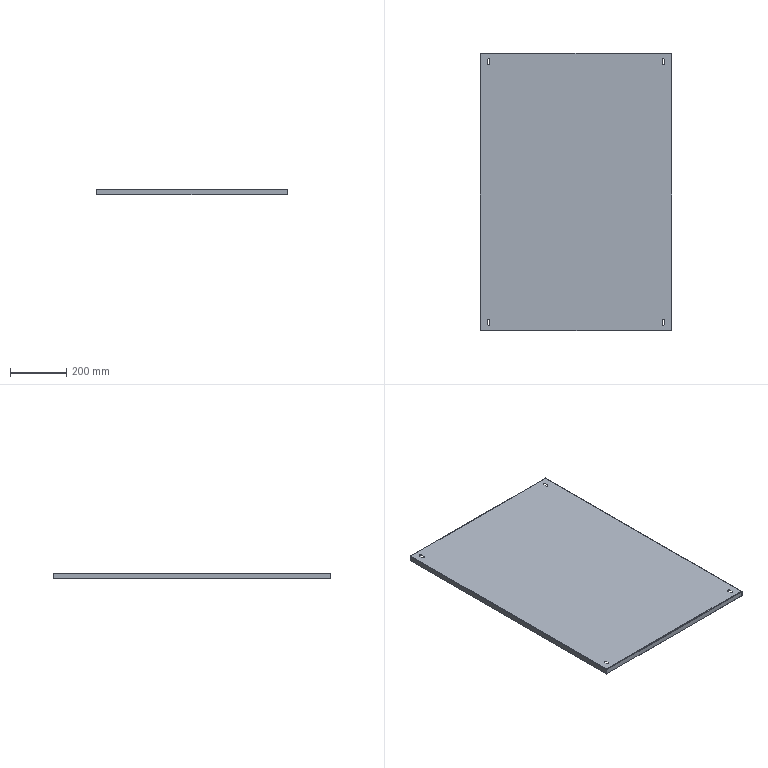Part | STEP file | Electrical Cabinet Base Plate | 1 solid | 50 faces | box 680 x 985 x 20 mm | volume 1454613 mm3 | plane 34 | cylinder 16 | commonest cylinder face diameters 10 x8 0.2 x4 4.2 x4
STEP:
#1=CARTESIAN_POINT('',(327.279,-432.271,-2.));
#2=VERTEX_POINT('',#1);
#3=CARTESIAN_POINT('',(327.279,548.529,-2.));
#4=VERTEX_POINT('',#3);
#5=CARTESIAN_POINT('',(327.279,0.,-2.));
#6=DIRECTION('',(0.,1.,0.));
#7=VECTOR('',#6,1000.);
#8=LINE('',#5,#7);
#9=EDGE_CURVE('',#2,#4,#8,.T.);
#10=ORIENTED_EDGE('',*,*,#9,.F.);
#11=CARTESIAN_POINT('',(-348.521,-432.271,-2.));
#12=VERTEX_POINT('',#11);
#13=CARTESIAN_POINT('',(0.,-432.271,-2.));
#14=DIRECTION('',(1.,0.,0.));
#15=VECTOR('',#14,1000.);
#16=LINE('',#13,#15);
#17=EDGE_CURVE('',#12,#2,#16,.T.);
#18=ORIENTED_EDGE('',*,*,#17,.F.);
#19=CARTESIAN_POINT('',(-348.521,548.529,-2.));
#20=VERTEX_POINT('',#19);
#21=CARTESIAN_POINT('',(-348.521,0.,-2.));
#22=DIRECTION('',(0.,-1.,0.));
#23=VECTOR('',#22,1000.);
#24=LINE('',#21,#23);
#25=EDGE_CURVE('',#20,#12,#24,.T.);
#26=ORIENTED_EDGE('',*,*,#25,.F.);
#27=CARTESIAN_POINT('',(0.,548.529,-2.));
#28=DIRECTION('',(-1.,0.,0.));
#29=VECTOR('',#28,1000.);
#30=LINE('',#27,#29);
#31=EDGE_CURVE('',#4,#20,#30,.T.);
#32=ORIENTED_EDGE('',*,*,#31,.F.);
#33=EDGE_LOOP('',(#10,#18,#26,#32));
#34=FACE_OUTER_BOUND('',#33,.T.);
#35=CARTESIAN_POINT('',(294.379,-399.371,-2.));
#36=VERTEX_POINT('',#35);
#37=CARTESIAN_POINT('',(304.379,-399.371,-2.));
#38=VERTEX_POINT('',#37);
#39=CARTESIAN_POINT('',(299.379,-399.371,-2.));
#40=DIRECTION('',(0.,0.,-1.));
#41=DIRECTION('',(1.,0.,0.));
#42=AXIS2_PLACEMENT_3D('',#39,#40,#41);
#43=CIRCLE('',#42,5.);
#44=EDGE_CURVE('',#36,#38,#43,.T.);
#45=ORIENTED_EDGE('',*,*,#44,.F.);
#46=CARTESIAN_POINT('',(294.379,-409.371,-2.));
#47=VERTEX_POINT('',#46);
#48=CARTESIAN_POINT('',(294.379,0.,-2.));
#49=DIRECTION('',(0.,1.,0.));
#50=VECTOR('',#49,1000.);
#51=LINE('',#48,#50);
#52=EDGE_CURVE('',#47,#36,#51,.T.);
#53=ORIENTED_EDGE('',*,*,#52,.F.);
#54=CARTESIAN_POINT('',(304.379,-409.371,-2.));
#55=VERTEX_POINT('',#54);
#56=CARTESIAN_POINT('',(299.379,-409.371,-2.));
#57=DIRECTION('',(0.,0.,-1.));
#58=DIRECTION('',(1.,0.,0.));
#59=AXIS2_PLACEMENT_3D('',#56,#57,#58);
#60=CIRCLE('',#59,5.);
#61=EDGE_CURVE('',#55,#47,#60,.T.);
#62=ORIENTED_EDGE('',*,*,#61,.F.);
#63=CARTESIAN_POINT('',(304.379,0.,-2.));
#64=DIRECTION('',(0.,-1.,0.));
#65=VECTOR('',#64,1000.);
#66=LINE('',#63,#65);
#67=EDGE_CURVE('',#38,#55,#66,.T.);
#68=ORIENTED_EDGE('',*,*,#67,.F.);
#69=EDGE_LOOP('',(#45,#53,#62,#68));
#70=FACE_BOUND('',#69,.T.);
#71=CARTESIAN_POINT('',(-325.621,-399.371,-2.));
#72=VERTEX_POINT('',#71);
#73=CARTESIAN_POINT('',(-315.621,-399.371,-2.));
#74=VERTEX_POINT('',#73);
#75=CARTESIAN_POINT('',(-320.621,-399.371,-2.));
#76=DIRECTION('',(0.,0.,-1.));
#77=DIRECTION('',(1.,0.,0.));
#78=AXIS2_PLACEMENT_3D('',#75,#76,#77);
#79=CIRCLE('',#78,5.);
#80=EDGE_CURVE('',#72,#74,#79,.T.);
#81=ORIENTED_EDGE('',*,*,#80,.F.);
#82=CARTESIAN_POINT('',(-325.621,-409.371,-2.));
#83=VERTEX_POINT('',#82);
#84=CARTESIAN_POINT('',(-325.621,0.,-2.));
#85=DIRECTION('',(0.,1.,0.));
#86=VECTOR('',#85,1000.);
#87=LINE('',#84,#86);
#88=EDGE_CURVE('',#83,#72,#87,.T.);
#89=ORIENTED_EDGE('',*,*,#88,.F.);
#90=CARTESIAN_POINT('',(-315.621,-409.371,-2.));
#91=VERTEX_POINT('',#90);
#92=CARTESIAN_POINT('',(-320.621,-409.371,-2.));
#93=DIRECTION('',(0.,0.,-1.));
#94=DIRECTION('',(1.,0.,0.));
#95=AXIS2_PLACEMENT_3D('',#92,#93,#94);
#96=CIRCLE('',#95,5.);
#97=EDGE_CURVE('',#91,#83,#96,.T.);
#98=ORIENTED_EDGE('',*,*,#97,.F.);
#99=CARTESIAN_POINT('',(-315.621,0.,-2.));
#100=DIRECTION('',(0.,-1.,0.));
#101=VECTOR('',#100,1000.);
#102=LINE('',#99,#101);
#103=EDGE_CURVE('',#74,#91,#102,.T.);
#104=ORIENTED_EDGE('',*,*,#103,.F.);
#105=EDGE_LOOP('',(#81,#89,#98,#104));
#106=FACE_BOUND('',#105,.T.);
#107=CARTESIAN_POINT('',(-325.621,525.629,-2.));
#108=VERTEX_POINT('',#107);
#109=CARTESIAN_POINT('',(-315.621,525.629,-2.));
#110=VERTEX_POINT('',#109);
#111=CARTESIAN_POINT('',(-320.621,525.629,-2.));
#112=DIRECTION('',(0.,0.,-1.));
#113=DIRECTION('',(1.,0.,0.));
#114=AXIS2_PLACEMENT_3D('',#111,#112,#113);
#115=CIRCLE('',#114,5.);
#116=EDGE_CURVE('',#108,#110,#115,.T.);
#117=ORIENTED_EDGE('',*,*,#116,.F.);
#118=CARTESIAN_POINT('',(-325.621,515.629,-2.));
#119=VERTEX_POINT('',#118);
#120=CARTESIAN_POINT('',(-325.621,0.,-2.));
#121=DIRECTION('',(0.,1.,0.));
#122=VECTOR('',#121,1000.);
#123=LINE('',#120,#122);
#124=EDGE_CURVE('',#119,#108,#123,.T.);
#125=ORIENTED_EDGE('',*,*,#124,.F.);
#126=CARTESIAN_POINT('',(-315.621,515.629,-2.));
#127=VERTEX_POINT('',#126);
#128=CARTESIAN_POINT('',(-320.621,515.629,-2.));
#129=DIRECTION('',(0.,0.,-1.));
#130=DIRECTION('',(1.,0.,0.));
#131=AXIS2_PLACEMENT_3D('',#128,#129,#130);
#132=CIRCLE('',#131,5.);
#133=EDGE_CURVE('',#127,#119,#132,.T.);
#134=ORIENTED_EDGE('',*,*,#133,.F.);
#135=CARTESIAN_POINT('',(-315.621,0.,-2.));
#136=DIRECTION('',(0.,-1.,0.));
#137=VECTOR('',#136,1000.);
#138=LINE('',#135,#137);
#139=EDGE_CURVE('',#110,#127,#138,.T.);
#140=ORIENTED_EDGE('',*,*,#139,.F.);
#141=EDGE_LOOP('',(#117,#125,#134,#140));
#142=FACE_BOUND('',#141,.T.);
#143=CARTESIAN_POINT('',(294.379,525.629,-2.));
#144=VERTEX_POINT('',#143);
#145=CARTESIAN_POINT('',(304.379,525.629,-2.));
#146=VERTEX_POINT('',#145);
#147=CARTESIAN_POINT('',(299.379,525.629,-2.));
#148=DIRECTION('',(0.,0.,-1.));
#149=DIRECTION('',(1.,0.,0.));
#150=AXIS2_PLACEMENT_3D('',#147,#148,#149);
#151=CIRCLE('',#150,5.);
#152=EDGE_CURVE('',#144,#146,#151,.T.);
#153=ORIENTED_EDGE('',*,*,#152,.F.);
#154=CARTESIAN_POINT('',(294.379,515.629,-2.));
#155=VERTEX_POINT('',#154);
#156=CARTESIAN_POINT('',(294.379,0.,-2.));
#157=DIRECTION('',(0.,1.,0.));
#158=VECTOR('',#157,1000.);
#159=LINE('',#156,#158);
#160=EDGE_CURVE('',#155,#144,#159,.T.);
#161=ORIENTED_EDGE('',*,*,#160,.F.);
#162=CARTESIAN_POINT('',(304.379,515.629,-2.));
#163=VERTEX_POINT('',#162);
#164=CARTESIAN_POINT('',(299.379,515.629,-2.));
#165=DIRECTION('',(0.,0.,-1.));
#166=DIRECTION('',(1.,0.,0.));
#167=AXIS2_PLACEMENT_3D('',#164,#165,#166);
#168=CIRCLE('',#167,5.);
#169=EDGE_CURVE('',#163,#155,#168,.T.);
#170=ORIENTED_EDGE('',*,*,#169,.F.);
#171=CARTESIAN_POINT('',(304.379,0.,-2.));
#172=DIRECTION('',(0.,-1.,0.));
#173=VECTOR('',#172,1000.);
#174=LINE('',#171,#173);
#175=EDGE_CURVE('',#146,#163,#174,.T.);
#176=ORIENTED_EDGE('',*,*,#175,.F.);
#177=EDGE_LOOP('',(#153,#161,#170,#176));
#178=FACE_BOUND('',#177,.T.);
#179=CARTESIAN_POINT('',(0.,0.,-2.));
#180=DIRECTION('',(0.,0.,1.));
#181=DIRECTION('',(1.,0.,0.));
#182=AXIS2_PLACEMENT_3D('',#179,#180,#181);
#183=PLANE('',#182);
#184=ADVANCED_FACE('',(#34,#70,#106,#142,#178),#183,.F.);
#185=CARTESIAN_POINT('',(-348.521,548.629,-2.1));
#186=VERTEX_POINT('',#185);
#187=CARTESIAN_POINT('',(-348.521,548.529,-2.1));
#188=DIRECTION('',(1.,0.,0.));
#189=DIRECTION('',(0.,0.,-1.));
#190=AXIS2_PLACEMENT_3D('',#187,#188,#189);
#191=CIRCLE('',#190,0.1);
#192=EDGE_CURVE('',#186,#20,#191,.T.);
#193=ORIENTED_EDGE('',*,*,#192,.F.);
#194=CARTESIAN_POINT('',(327.279,548.629,-2.1));
#195=VERTEX_POINT('',#194);
#196=CARTESIAN_POINT('',(327.279,548.629,-2.1));
#197=DIRECTION('',(-1.,0.,0.));
#198=VECTOR('',#197,1000.);
#199=LINE('',#196,#198);
#200=EDGE_CURVE('',#195,#186,#199,.T.);
#201=ORIENTED_EDGE('',*,*,#200,.F.);
#202=CARTESIAN_POINT('',(327.279,548.529,-2.1));
#203=DIRECTION('',(1.,0.,0.));
#204=DIRECTION('',(0.,0.,-1.));
#205=AXIS2_PLACEMENT_3D('',#202,#203,#204);
#206=CIRCLE('',#205,0.1);
#207=EDGE_CURVE('',#195,#4,#206,.T.);
#208=ORIENTED_EDGE('',*,*,#207,.T.);
#209=ORIENTED_EDGE('',*,*,#31,.T.);
#210=EDGE_LOOP('',(#193,#201,#208,#209));
#211=FACE_OUTER_BOUND('',#210,.T.);
#212=CARTESIAN_POINT('',(327.279,548.529,-2.1));
#213=DIRECTION('',(1.,0.,0.));
#214=DIRECTION('',(0.,0.,-1.));
#215=AXIS2_PLACEMENT_3D('',#212,#213,#214);
#216=CYLINDRICAL_SURFACE('',#215,0.1);
#217=ADVANCED_FACE('',(#211),#216,.F.);
#218=CARTESIAN_POINT('',(327.279,-434.369,-2.));
#219=VERTEX_POINT('',#218);
#220=CARTESIAN_POINT('',(327.279,-434.371,-2.));
#221=DIRECTION('',(0.,-1.,0.));
#222=VECTOR('',#221,1000.);
#223=LINE('',#220,#222);
#224=EDGE_CURVE('',#2,#219,#223,.T.);
#225=ORIENTED_EDGE('',*,*,#224,.F.);
#226=ORIENTED_EDGE('',*,*,#9,.T.);
#227=CARTESIAN_POINT('',(327.279,550.626,-2.));
#228=VERTEX_POINT('',#227);
#229=CARTESIAN_POINT('',(327.279,-434.371,-2.));
#230=DIRECTION('',(0.,-1.,0.));
#231=VECTOR('',#230,1000.);
#232=LINE('',#229,#231);
#233=EDGE_CURVE('',#228,#4,#232,.T.);
#234=ORIENTED_EDGE('',*,*,#233,.F.);
#235=CARTESIAN_POINT('',(327.279,550.629,-2.));
#236=VERTEX_POINT('',#235);
#237=CARTESIAN_POINT('',(327.279,550.629,-2.));
#238=DIRECTION('',(0.,-1.,0.));
#239=VECTOR('',#238,1000.);
#240=LINE('',#237,#239);
#241=EDGE_CURVE('',#236,#228,#240,.T.);
#242=ORIENTED_EDGE('',*,*,#241,.F.);
#243=CARTESIAN_POINT('',(327.379,550.629,-2.1));
#244=VERTEX_POINT('',#243);
#245=CARTESIAN_POINT('',(327.279,550.629,-2.1));
#246=DIRECTION('',(0.,-1.,0.));
#247=DIRECTION('',(0.,0.,-1.));
#248=AXIS2_PLACEMENT_3D('',#245,#246,#247);
#249=CIRCLE('',#248,0.1);
#250=EDGE_CURVE('',#244,#236,#249,.T.);
#251=ORIENTED_EDGE('',*,*,#250,.F.);
#252=CARTESIAN_POINT('',(327.379,-434.371,-2.1));
#253=VERTEX_POINT('',#252);
#254=CARTESIAN_POINT('',(327.379,-434.371,-2.1));
#255=DIRECTION('',(0.,1.,0.));
#256=VECTOR('',#255,1000.);
#257=LINE('',#254,#256);
#258=EDGE_CURVE('',#253,#244,#257,.T.);
#259=ORIENTED_EDGE('',*,*,#258,.F.);
#260=CARTESIAN_POINT('',(327.279,-434.371,-2.));
#261=VERTEX_POINT('',#260);
#262=CARTESIAN_POINT('',(327.279,-434.371,-2.1));
#263=DIRECTION('',(0.,-1.,0.));
#264=DIRECTION('',(0.,0.,-1.));
#265=AXIS2_PLACEMENT_3D('',#262,#263,#264);
#266=CIRCLE('',#265,0.1);
#267=EDGE_CURVE('',#253,#261,#266,.T.);
#268=ORIENTED_EDGE('',*,*,#267,.T.);
#269=CARTESIAN_POINT('',(327.279,-432.271,-2.));
#270=DIRECTION('',(0.,-1.,0.));
#271=VECTOR('',#270,1000.);
#272=LINE('',#269,#271);
#273=EDGE_CURVE('',#219,#261,#272,.T.);
#274=ORIENTED_EDGE('',*,*,#273,.F.);
#275=EDGE_LOOP('',(#225,#226,#234,#242,#251,#259,#268,#274));
#276=FACE_OUTER_BOUND('',#275,.T.);
#277=CARTESIAN_POINT('',(327.279,-434.371,-2.1));
#278=DIRECTION('',(0.,-1.,0.));
#279=DIRECTION('',(0.,0.,-1.));
#280=AXIS2_PLACEMENT_3D('',#277,#278,#279);
#281=CYLINDRICAL_SURFACE('',#280,0.1);
#282=ADVANCED_FACE('',(#276),#281,.F.);
#283=CARTESIAN_POINT('',(327.279,-432.371,-2.1));
#284=VERTEX_POINT('',#283);
#285=CARTESIAN_POINT('',(327.279,-432.271,-2.1));
#286=DIRECTION('',(-1.,0.,0.));
#287=DIRECTION('',(0.,0.,1.));
#288=AXIS2_PLACEMENT_3D('',#285,#286,#287);
#289=CIRCLE('',#288,0.1);
#290=EDGE_CURVE('',#284,#2,#289,.T.);
#291=ORIENTED_EDGE('',*,*,#290,.F.);
#292=CARTESIAN_POINT('',(-348.521,-432.371,-2.1));
#293=VERTEX_POINT('',#292);
#294=CARTESIAN_POINT('',(-348.521,-432.371,-2.1));
#295=DIRECTION('',(1.,0.,0.));
#296=VECTOR('',#295,1000.);
#297=LINE('',#294,#296);
#298=EDGE_CURVE('',#293,#284,#297,.T.);
#299=ORIENTED_EDGE('',*,*,#298,.F.);
#300=CARTESIAN_POINT('',(-348.521,-432.271,-2.1));
#301=DIRECTION('',(-1.,0.,0.));
#302=DIRECTION('',(0.,0.,1.));
#303=AXIS2_PLACEMENT_3D('',#300,#301,#302);
#304=CIRCLE('',#303,0.1);
#305=EDGE_CURVE('',#293,#12,#304,.T.);
#306=ORIENTED_EDGE('',*,*,#305,.T.);
#307=ORIENTED_EDGE('',*,*,#17,.T.);
#308=EDGE_LOOP('',(#291,#299,#306,#307));
#309=FACE_OUTER_BOUND('',#308,.T.);
#310=CARTESIAN_POINT('',(-348.521,-432.271,-2.1));
#311=DIRECTION('',(-1.,0.,0.));
#312=DIRECTION('',(0.,0.,1.));
#313=AXIS2_PLACEMENT_3D('',#310,#311,#312);
#314=CYLINDRICAL_SURFACE('',#313,0.1);
#315=ADVANCED_FACE('',(#309),#314,.F.);
#316=CARTESIAN_POINT('',(-348.521,550.626,-2.));
#317=VERTEX_POINT('',#316);
#318=CARTESIAN_POINT('',(-348.521,548.529,-2.));
#319=DIRECTION('',(0.,1.,0.));
#320=VECTOR('',#319,1000.);
#321=LINE('',#318,#320);
#322=EDGE_CURVE('',#20,#317,#321,.T.);
#323=ORIENTED_EDGE('',*,*,#322,.F.);
#324=ORIENTED_EDGE('',*,*,#25,.T.);
#325=CARTESIAN_POINT('',(-348.521,-434.369,-2.));
#326=VERTEX_POINT('',#325);
#327=CARTESIAN_POINT('',(-348.521,550.629,-2.));
#328=DIRECTION('',(0.,1.,0.));
#329=VECTOR('',#328,1000.);
#330=LINE('',#327,#329);
#331=EDGE_CURVE('',#326,#12,#330,.T.);
#332=ORIENTED_EDGE('',*,*,#331,.F.);
#333=CARTESIAN_POINT('',(-348.521,-434.371,-2.));
#334=VERTEX_POINT('',#333);
#335=CARTESIAN_POINT('',(-348.521,-434.371,-2.));
#336=DIRECTION('',(0.,1.,0.));
#337=VECTOR('',#336,1000.);
#338=LINE('',#335,#337);
#339=EDGE_CURVE('',#334,#326,#338,.T.);
#340=ORIENTED_EDGE('',*,*,#339,.F.);
#341=CARTESIAN_POINT('',(-348.621,-434.371,-2.1));
#342=VERTEX_POINT('',#341);
#343=CARTESIAN_POINT('',(-348.521,-434.371,-2.1));
#344=DIRECTION('',(0.,1.,0.));
#345=DIRECTION('',(0.,0.,1.));
#346=AXIS2_PLACEMENT_3D('',#343,#344,#345);
#347=CIRCLE('',#346,0.1);
#348=EDGE_CURVE('',#342,#334,#347,.T.);
#349=ORIENTED_EDGE('',*,*,#348,.F.);
#350=CARTESIAN_POINT('',(-348.621,550.629,-2.1));
#351=VERTEX_POINT('',#350);
#352=CARTESIAN_POINT('',(-348.621,550.629,-2.1));
#353=DIRECTION('',(0.,-1.,0.));
#354=VECTOR('',#353,1000.);
#355=LINE('',#352,#354);
#356=EDGE_CURVE('',#351,#342,#355,.T.);
#357=ORIENTED_EDGE('',*,*,#356,.F.);
#358=CARTESIAN_POINT('',(-348.521,550.629,-2.));
#359=VERTEX_POINT('',#358);
#360=CARTESIAN_POINT('',(-348.521,550.629,-2.1));
#361=DIRECTION('',(0.,1.,0.));
#362=DIRECTION('',(0.,0.,1.));
#363=AXIS2_PLACEMENT_3D('',#360,#361,#362);
#364=CIRCLE('',#363,0.1);
#365=EDGE_CURVE('',#351,#359,#364,.T.);
#366=ORIENTED_EDGE('',*,*,#365,.T.);
#367=CARTESIAN_POINT('',(-348.521,548.529,-2.));
#368=DIRECTION('',(0.,1.,0.));
#369=VECTOR('',#368,1000.);
#370=LINE('',#367,#369);
#371=EDGE_CURVE('',#317,#359,#370,.T.);
#372=ORIENTED_EDGE('',*,*,#371,.F.);
#373=EDGE_LOOP('',(#323,#324,#332,#340,#349,#357,#366,#372));
#374=FACE_OUTER_BOUND('',#373,.T.);
#375=CARTESIAN_POINT('',(-348.521,550.629,-2.1));
#376=DIRECTION('',(0.,1.,0.));
#377=DIRECTION('',(0.,0.,1.));
#378=AXIS2_PLACEMENT_3D('',#375,#376,#377);
#379=CYLINDRICAL_SURFACE('',#378,0.1);
#380=ADVANCED_FACE('',(#374),#379,.F.);
#381=CARTESIAN_POINT('',(304.379,-399.371,0.));
#382=VERTEX_POINT('',#381);
#383=CARTESIAN_POINT('',(304.379,-399.371,-2.));
#384=DIRECTION('',(0.,0.,1.));
#385=VECTOR('',#384,1000.);
#386=LINE('',#383,#385);
#387=EDGE_CURVE('',#38,#382,#386,.T.);
#388=ORIENTED_EDGE('',*,*,#387,.F.);
#389=ORIENTED_EDGE('',*,*,#67,.T.);
#390=CARTESIAN_POINT('',(304.379,-409.371,0.));
#391=VERTEX_POINT('',#390);
#392=CARTESIAN_POINT('',(304.379,-409.371,-2.));
#393=DIRECTION('',(0.,0.,-1.));
#394=VECTOR('',#393,1000.);
#395=LINE('',#392,#394);
#396=EDGE_CURVE('',#391,#55,#395,.T.);
#397=ORIENTED_EDGE('',*,*,#396,.F.);
#398=CARTESIAN_POINT('',(304.379,-399.371,0.));
#399=DIRECTION('',(0.,-1.,0.));
#400=VECTOR('',#399,1000.);
#401=LINE('',#398,#400);
#402=EDGE_CURVE('',#382,#391,#401,.T.);
#403=ORIENTED_EDGE('',*,*,#402,.F.);
#404=EDGE_LOOP('',(#388,#389,#397,#403));
#405=FACE_OUTER_BOUND('',#404,.T.);
#406=CARTESIAN_POINT('',(304.379,-399.371,-2.));
#407=DIRECTION('',(1.,0.,0.));
#408=DIRECTION('',(0.,0.,-1.));
#409=AXIS2_PLACEMENT_3D('',#406,#407,#408);
#410=PLANE('',#409);
#411=ADVANCED_FACE('',(#405),#410,.F.);
#412=CARTESIAN_POINT('',(294.379,-399.371,0.));
#413=VERTEX_POINT('',#412);
#414=CARTESIAN_POINT('',(294.379,-399.371,-2.));
#415=DIRECTION('',(0.,0.,1.));
#416=VECTOR('',#415,1000.);
#417=LINE('',#414,#416);
#418=EDGE_CURVE('',#36,#413,#417,.T.);
#419=ORIENTED_EDGE('',*,*,#418,.F.);
#420=ORIENTED_EDGE('',*,*,#44,.T.);
#421=ORIENTED_EDGE('',*,*,#387,.T.);
#422=CARTESIAN_POINT('',(299.379,-399.371,0.));
#423=DIRECTION('',(0.,0.,-1.));
#424=DIRECTION('',(1.,0.,0.));
#425=AXIS2_PLACEMENT_3D('',#422,#423,#424);
#426=CIRCLE('',#425,5.);
#427=EDGE_CURVE('',#413,#382,#426,.T.);
#428=ORIENTED_EDGE('',*,*,#427,.F.);
#429=EDGE_LOOP('',(#419,#420,#421,#428));
#430=FACE_OUTER_BOUND('',#429,.T.);
#431=CARTESIAN_POINT('',(299.379,-399.371,-2.));
#432=DIRECTION('',(0.,0.,1.));
#433=DIRECTION('',(1.,0.,0.));
#434=AXIS2_PLACEMENT_3D('',#431,#432,#433);
#435=CYLINDRICAL_SURFACE('',#434,5.);
#436=ADVANCED_FACE('',(#430),#435,.F.);
#437=CARTESIAN_POINT('',(294.379,-409.371,0.));
#438=VERTEX_POINT('',#437);
#439=CARTESIAN_POINT('',(294.379,-409.371,-2.));
#440=DIRECTION('',(0.,0.,1.));
#441=VECTOR('',#440,1000.);
#442=LINE('',#439,#441);
#443=EDGE_CURVE('',#47,#438,#442,.T.);
#444=ORIENTED_EDGE('',*,*,#443,.F.);
#445=ORIENTED_EDGE('',*,*,#52,.T.);
#446=ORIENTED_EDGE('',*,*,#418,.T.);
#447=CARTESIAN_POINT('',(294.379,-399.371,0.));
#448=DIRECTION('',(0.,1.,0.));
#449=VECTOR('',#448,1000.);
#450=LINE('',#447,#449);
#451=EDGE_CURVE('',#438,#413,#450,.T.);
#452=ORIENTED_EDGE('',*,*,#451,.F.);
#453=EDGE_LOOP('',(#444,#445,#446,#452));
#454=FACE_OUTER_BOUND('',#453,.T.);
#455=CARTESIAN_POINT('',(294.379,-399.371,-2.));
#456=DIRECTION('',(-1.,0.,0.));
#457=DIRECTION('',(0.,0.,1.));
#458=AXIS2_PLACEMENT_3D('',#455,#456,#457);
#459=PLANE('',#458);
#460=ADVANCED_FACE('',(#454),#459,.F.);
#461=ORIENTED_EDGE('',*,*,#396,.T.);
#462=ORIENTED_EDGE('',*,*,#61,.T.);
#463=ORIENTED_EDGE('',*,*,#443,.T.);
#464=CARTESIAN_POINT('',(299.379,-409.371,0.));
#465=DIRECTION('',(0.,0.,-1.));
#466=DIRECTION('',(1.,0.,0.));
#467=AXIS2_PLACEMENT_3D('',#464,#465,#466);
#468=CIRCLE('',#467,5.);
#469=EDGE_CURVE('',#391,#438,#468,.T.);
#470=ORIENTED_EDGE('',*,*,#469,.F.);
#471=EDGE_LOOP('',(#461,#462,#463,#470));
#472=FACE_OUTER_BOUND('',#471,.T.);
#473=CARTESIAN_POINT('',(299.379,-409.371,-2.));
#474=DIRECTION('',(0.,0.,1.));
#475=DIRECTION('',(1.,0.,0.));
#476=AXIS2_PLACEMENT_3D('',#473,#474,#475);
#477=CYLINDRICAL_SURFACE('',#476,5.);
#478=ADVANCED_FACE('',(#472),#477,.F.);
#479=CARTESIAN_POINT('',(-315.621,-399.371,0.));
#480=VERTEX_POINT('',#479);
#481=CARTESIAN_POINT('',(-315.621,-399.371,-2.));
#482=DIRECTION('',(0.,0.,1.));
#483=VECTOR('',#482,1000.);
#484=LINE('',#481,#483);
#485=EDGE_CURVE('',#74,#480,#484,.T.);
#486=ORIENTED_EDGE('',*,*,#485,.F.);
#487=ORIENTED_EDGE('',*,*,#103,.T.);
#488=CARTESIAN_POINT('',(-315.621,-409.371,0.));
#489=VERTEX_POINT('',#488);
#490=CARTESIAN_POINT('',(-315.621,-409.371,-2.));
#491=DIRECTION('',(0.,0.,-1.));
#492=VECTOR('',#491,1000.);
#493=LINE('',#490,#492);
#494=EDGE_CURVE('',#489,#91,#493,.T.);
#495=ORIENTED_EDGE('',*,*,#494,.F.);
#496=CARTESIAN_POINT('',(-315.621,-399.371,0.));
#497=DIRECTION('',(0.,-1.,0.));
#498=VECTOR('',#497,1000.);
#499=LINE('',#496,#498);
#500=EDGE_CURVE('',#480,#489,#499,.T.);
#501=ORIENTED_EDGE('',*,*,#500,.F.);
#502=EDGE_LOOP('',(#486,#487,#495,#501));
#503=FACE_OUTER_BOUND('',#502,.T.);
#504=CARTESIAN_POINT('',(-315.621,-399.371,-2.));
#505=DIRECTION('',(1.,0.,0.));
#506=DIRECTION('',(0.,0.,-1.));
#507=AXIS2_PLACEMENT_3D('',#504,#505,#506);
#508=PLANE('',#507);
#509=ADVANCED_FACE('',(#503),#508,.F.);
#510=CARTESIAN_POINT('',(-325.621,-399.371,0.));
#511=VERTEX_POINT('',#510);
#512=CARTESIAN_POINT('',(-325.621,-399.371,-2.));
#513=DIRECTION('',(0.,0.,1.));
#514=VECTOR('',#513,1000.);
#515=LINE('',#512,#514);
#516=EDGE_CURVE('',#72,#511,#515,.T.);
#517=ORIENTED_EDGE('',*,*,#516,.F.);
#518=ORIENTED_EDGE('',*,*,#80,.T.);
#519=ORIENTED_EDGE('',*,*,#485,.T.);
#520=CARTESIAN_POINT('',(-320.621,-399.371,0.));
#521=DIRECTION('',(0.,0.,-1.));
#522=DIRECTION('',(1.,0.,0.));
#523=AXIS2_PLACEMENT_3D('',#520,#521,#522);
#524=CIRCLE('',#523,5.);
#525=EDGE_CURVE('',#511,#480,#524,.T.);
#526=ORIENTED_EDGE('',*,*,#525,.F.);
#527=EDGE_LOOP('',(#517,#518,#519,#526));
#528=FACE_OUTER_BOUND('',#527,.T.);
#529=CARTESIAN_POINT('',(-320.621,-399.371,-2.));
#530=DIRECTION('',(0.,0.,1.));
#531=DIRECTION('',(1.,0.,0.));
#532=AXIS2_PLACEMENT_3D('',#529,#530,#531);
#533=CYLINDRICAL_SURFACE('',#532,5.);
#534=ADVANCED_FACE('',(#528),#533,.F.);
#535=CARTESIAN_POINT('',(-325.621,-409.371,0.));
#536=VERTEX_POINT('',#535);
#537=CARTESIAN_POINT('',(-325.621,-409.371,-2.));
#538=DIRECTION('',(0.,0.,1.));
#539=VECTOR('',#538,1000.);
#540=LINE('',#537,#539);
#541=EDGE_CURVE('',#83,#536,#540,.T.);
#542=ORIENTED_EDGE('',*,*,#541,.F.);
#543=ORIENTED_EDGE('',*,*,#88,.T.);
#544=ORIENTED_EDGE('',*,*,#516,.T.);
#545=CARTESIAN_POINT('',(-325.621,-399.371,0.));
#546=DIRECTION('',(0.,1.,0.));
#547=VECTOR('',#546,1000.);
#548=LINE('',#545,#547);
#549=EDGE_CURVE('',#536,#511,#548,.T.);
#550=ORIENTED_EDGE('',*,*,#549,.F.);
#551=EDGE_LOOP('',(#542,#543,#544,#550));
#552=FACE_OUTER_BOUND('',#551,.T.);
#553=CARTESIAN_POINT('',(-325.621,-399.371,-2.));
#554=DIRECTION('',(-1.,0.,0.));
#555=DIRECTION('',(0.,0.,1.));
#556=AXIS2_PLACEMENT_3D('',#553,#554,#555);
#557=PLANE('',#556);
#558=ADVANCED_FACE('',(#552),#557,.F.);
#559=ORIENTED_EDGE('',*,*,#494,.T.);
#560=ORIENTED_EDGE('',*,*,#97,.T.);
#561=ORIENTED_EDGE('',*,*,#541,.T.);
#562=CARTESIAN_POINT('',(-320.621,-409.371,0.));
#563=DIRECTION('',(0.,0.,-1.));
#564=DIRECTION('',(1.,0.,0.));
#565=AXIS2_PLACEMENT_3D('',#562,#563,#564);
#566=CIRCLE('',#565,5.);
#567=EDGE_CURVE('',#489,#536,#566,.T.);
#568=ORIENTED_EDGE('',*,*,#567,.F.);
#569=EDGE_LOOP('',(#559,#560,#561,#568));
#570=FACE_OUTER_BOUND('',#569,.T.);
#571=CARTESIAN_POINT('',(-320.621,-409.371,-2.));
#572=DIRECTION('',(0.,0.,1.));
#573=DIRECTION('',(1.,0.,0.));
#574=AXIS2_PLACEMENT_3D('',#571,#572,#573);
#575=CYLINDRICAL_SURFACE('',#574,5.);
#576=ADVANCED_FACE('',(#570),#575,.F.);
#577=CARTESIAN_POINT('',(-315.621,525.629,0.));
#578=VERTEX_POINT('',#577);
#579=CARTESIAN_POINT('',(-315.621,525.629,-2.));
#580=DIRECTION('',(0.,0.,1.));
#581=VECTOR('',#580,1000.);
#582=LINE('',#579,#581);
#583=EDGE_CURVE('',#110,#578,#582,.T.);
#584=ORIENTED_EDGE('',*,*,#583,.F.);
#585=ORIENTED_EDGE('',*,*,#139,.T.);
#586=CARTESIAN_POINT('',(-315.621,515.629,0.));
#587=VERTEX_POINT('',#586);
#588=CARTESIAN_POINT('',(-315.621,515.629,-2.));
#589=DIRECTION('',(0.,0.,-1.));
#590=VECTOR('',#589,1000.);
#591=LINE('',#588,#590);
#592=EDGE_CURVE('',#587,#127,#591,.T.);
#593=ORIENTED_EDGE('',*,*,#592,.F.);
#594=CARTESIAN_POINT('',(-315.621,525.629,0.));
#595=DIRECTION('',(0.,-1.,0.));
#596=VECTOR('',#595,1000.);
#597=LINE('',#594,#596);
#598=EDGE_CURVE('',#578,#587,#597,.T.);
#599=ORIENTED_EDGE('',*,*,#598,.F.);
#600=EDGE_LOOP('',(#584,#585,#593,#599));
#601=FACE_OUTER_BOUND('',#600,.T.);
#602=CARTESIAN_POINT('',(-315.621,525.629,-2.));
#603=DIRECTION('',(1.,0.,0.));
#604=DIRECTION('',(0.,0.,-1.));
#605=AXIS2_PLACEMENT_3D('',#602,#603,#604);
#606=PLANE('',#605);
#607=ADVANCED_FACE('',(#601),#606,.F.);
#608=CARTESIAN_POINT('',(-325.621,525.629,0.));
#609=VERTEX_POINT('',#608);
#610=CARTESIAN_POINT('',(-325.621,525.629,-2.));
#611=DIRECTION('',(0.,0.,1.));
#612=VECTOR('',#611,1000.);
#613=LINE('',#610,#612);
#614=EDGE_CURVE('',#108,#609,#613,.T.);
#615=ORIENTED_EDGE('',*,*,#614,.F.);
#616=ORIENTED_EDGE('',*,*,#116,.T.);
#617=ORIENTED_EDGE('',*,*,#583,.T.);
#618=CARTESIAN_POINT('',(-320.621,525.629,0.));
#619=DIRECTION('',(0.,0.,-1.));
#620=DIRECTION('',(1.,0.,0.));
#621=AXIS2_PLACEMENT_3D('',#618,#619,#620);
#622=CIRCLE('',#621,5.);
#623=EDGE_CURVE('',#609,#578,#622,.T.);
#624=ORIENTED_EDGE('',*,*,#623,.F.);
#625=EDGE_LOOP('',(#615,#616,#617,#624));
#626=FACE_OUTER_BOUND('',#625,.T.);
#627=CARTESIAN_POINT('',(-320.621,525.629,-2.));
#628=DIRECTION('',(0.,0.,1.));
#629=DIRECTION('',(1.,0.,0.));
#630=AXIS2_PLACEMENT_3D('',#627,#628,#629);
#631=CYLINDRICAL_SURFACE('',#630,5.);
#632=ADVANCED_FACE('',(#626),#631,.F.);
#633=CARTESIAN_POINT('',(-325.621,515.629,0.));
#634=VERTEX_POINT('',#633);
#635=CARTESIAN_POINT('',(-325.621,515.629,-2.));
#636=DIRECTION('',(0.,0.,1.));
#637=VECTOR('',#636,1000.);
#638=LINE('',#635,#637);
#639=EDGE_CURVE('',#119,#634,#638,.T.);
#640=ORIENTED_EDGE('',*,*,#639,.F.);
#641=ORIENTED_EDGE('',*,*,#124,.T.);
#642=ORIENTED_EDGE('',*,*,#614,.T.);
#643=CARTESIAN_POINT('',(-325.621,525.629,0.));
#644=DIRECTION('',(0.,1.,0.));
#645=VECTOR('',#644,1000.);
#646=LINE('',#643,#645);
#647=EDGE_CURVE('',#634,#609,#646,.T.);
#648=ORIENTED_EDGE('',*,*,#647,.F.);
#649=EDGE_LOOP('',(#640,#641,#642,#648));
#650=FACE_OUTER_BOUND('',#649,.T.);
#651=CARTESIAN_POINT('',(-325.621,525.629,-2.));
#652=DIRECTION('',(-1.,0.,0.));
#653=DIRECTION('',(0.,0.,1.));
#654=AXIS2_PLACEMENT_3D('',#651,#652,#653);
#655=PLANE('',#654);
#656=ADVANCED_FACE('',(#650),#655,.F.);
#657=ORIENTED_EDGE('',*,*,#592,.T.);
#658=ORIENTED_EDGE('',*,*,#133,.T.);
#659=ORIENTED_EDGE('',*,*,#639,.T.);
#660=CARTESIAN_POINT('',(-320.621,515.629,0.));
#661=DIRECTION('',(0.,0.,-1.));
#662=DIRECTION('',(1.,0.,0.));
#663=AXIS2_PLACEMENT_3D('',#660,#661,#662);
#664=CIRCLE('',#663,5.);
#665=EDGE_CURVE('',#587,#634,#664,.T.);
#666=ORIENTED_EDGE('',*,*,#665,.F.);
#667=EDGE_LOOP('',(#657,#658,#659,#666));
#668=FACE_OUTER_BOUND('',#667,.T.);
#669=CARTESIAN_POINT('',(-320.621,515.629,-2.));
#670=DIRECTION('',(0.,0.,1.));
#671=DIRECTION('',(1.,0.,0.));
#672=AXIS2_PLACEMENT_3D('',#669,#670,#671);
#673=CYLINDRICAL_SURFACE('',#672,5.);
#674=ADVANCED_FACE('',(#668),#673,.F.);
#675=CARTESIAN_POINT('',(304.379,525.629,0.));
#676=VERTEX_POINT('',#675);
#677=CARTESIAN_POINT('',(304.379,525.629,-2.));
#678=DIRECTION('',(0.,0.,1.));
#679=VECTOR('',#678,1000.);
#680=LINE('',#677,#679);
#681=EDGE_CURVE('',#146,#676,#680,.T.);
#682=ORIENTED_EDGE('',*,*,#681,.F.);
#683=ORIENTED_EDGE('',*,*,#175,.T.);
#684=CARTESIAN_POINT('',(304.379,515.629,0.));
#685=VERTEX_POINT('',#684);
#686=CARTESIAN_POINT('',(304.379,515.629,-2.));
#687=DIRECTION('',(0.,0.,-1.));
#688=VECTOR('',#687,1000.);
#689=LINE('',#686,#688);
#690=EDGE_CURVE('',#685,#163,#689,.T.);
#691=ORIENTED_EDGE('',*,*,#690,.F.);
#692=CARTESIAN_POINT('',(304.379,525.629,0.));
#693=DIRECTION('',(0.,-1.,0.));
#694=VECTOR('',#693,1000.);
#695=LINE('',#692,#694);
#696=EDGE_CURVE('',#676,#685,#695,.T.);
#697=ORIENTED_EDGE('',*,*,#696,.F.);
#698=EDGE_LOOP('',(#682,#683,#691,#697));
#699=FACE_OUTER_BOUND('',#698,.T.);
#700=CARTESIAN_POINT('',(304.379,525.629,-2.));
#701=DIRECTION('',(1.,0.,0.));
#702=DIRECTION('',(0.,0.,-1.));
#703=AXIS2_PLACEMENT_3D('',#700,#701,#702);
#704=PLANE('',#703);
#705=ADVANCED_FACE('',(#699),#704,.F.);
#706=CARTESIAN_POINT('',(294.379,525.629,0.));
#707=VERTEX_POINT('',#706);
#708=CARTESIAN_POINT('',(294.379,525.629,-2.));
#709=DIRECTION('',(0.,0.,1.));
#710=VECTOR('',#709,1000.);
#711=LINE('',#708,#710);
#712=EDGE_CURVE('',#144,#707,#711,.T.);
#713=ORIENTED_EDGE('',*,*,#712,.F.);
#714=ORIENTED_EDGE('',*,*,#152,.T.);
#715=ORIENTED_EDGE('',*,*,#681,.T.);
#716=CARTESIAN_POINT('',(299.379,525.629,0.));
#717=DIRECTION('',(0.,0.,-1.));
#718=DIRECTION('',(1.,0.,0.));
#719=AXIS2_PLACEMENT_3D('',#716,#717,#718);
#720=CIRCLE('',#719,5.);
#721=EDGE_CURVE('',#707,#676,#720,.T.);
#722=ORIENTED_EDGE('',*,*,#721,.F.);
#723=EDGE_LOOP('',(#713,#714,#715,#722));
#724=FACE_OUTER_BOUND('',#723,.T.);
#725=CARTESIAN_POINT('',(299.379,525.629,-2.));
#726=DIRECTION('',(0.,0.,1.));
#727=DIRECTION('',(1.,0.,0.));
#728=AXIS2_PLACEMENT_3D('',#725,#726,#727);
#729=CYLINDRICAL_SURFACE('',#728,5.);
#730=ADVANCED_FACE('',(#724),#729,.F.);
#731=CARTESIAN_POINT('',(294.379,515.629,0.));
#732=VERTEX_POINT('',#731);
#733=CARTESIAN_POINT('',(294.379,515.629,-2.));
#734=DIRECTION('',(0.,0.,1.));
#735=VECTOR('',#734,1000.);
#736=LINE('',#733,#735);
#737=EDGE_CURVE('',#155,#732,#736,.T.);
#738=ORIENTED_EDGE('',*,*,#737,.F.);
#739=ORIENTED_EDGE('',*,*,#160,.T.);
#740=ORIENTED_EDGE('',*,*,#712,.T.);
#741=CARTESIAN_POINT('',(294.379,525.629,0.));
#742=DIRECTION('',(0.,1.,0.));
#743=VECTOR('',#742,1000.);
#744=LINE('',#741,#743);
#745=EDGE_CURVE('',#732,#707,#744,.T.);
#746=ORIENTED_EDGE('',*,*,#745,.F.);
#747=EDGE_LOOP('',(#738,#739,#740,#746));
#748=FACE_OUTER_BOUND('',#747,.T.);
#749=CARTESIAN_POINT('',(294.379,525.629,-2.));
#750=DIRECTION('',(-1.,0.,0.));
#751=DIRECTION('',(0.,0.,1.));
#752=AXIS2_PLACEMENT_3D('',#749,#750,#751);
#753=PLANE('',#752);
#754=ADVANCED_FACE('',(#748),#753,.F.);
#755=ORIENTED_EDGE('',*,*,#690,.T.);
#756=ORIENTED_EDGE('',*,*,#169,.T.);
#757=ORIENTED_EDGE('',*,*,#737,.T.);
#758=CARTESIAN_POINT('',(299.379,515.629,0.));
#759=DIRECTION('',(0.,0.,-1.));
#760=DIRECTION('',(1.,0.,0.));
#761=AXIS2_PLACEMENT_3D('',#758,#759,#760);
#762=CIRCLE('',#761,5.);
#763=EDGE_CURVE('',#685,#732,#762,.T.);
#764=ORIENTED_EDGE('',*,*,#763,.F.);
#765=EDGE_LOOP('',(#755,#756,#757,#764));
#766=FACE_OUTER_BOUND('',#765,.T.);
#767=CARTESIAN_POINT('',(299.379,515.629,-2.));
#768=DIRECTION('',(0.,0.,1.));
#769=DIRECTION('',(1.,0.,0.));
#770=AXIS2_PLACEMENT_3D('',#767,#768,#769);
#771=CYLINDRICAL_SURFACE('',#770,5.);
#772=ADVANCED_FACE('',(#766),#771,.F.);
#773=CARTESIAN_POINT('',(-348.521,548.629,-20.));
#774=VERTEX_POINT('',#773);
#775=CARTESIAN_POINT('',(-348.521,548.629,0.));
#776=DIRECTION('',(0.,0.,-1.));
#777=VECTOR('',#776,1000.);
#778=LINE('',#775,#777);
#779=EDGE_CURVE('',#186,#774,#778,.T.);
#780=ORIENTED_EDGE('',*,*,#779,.T.);
#781=CARTESIAN_POINT('',(327.279,548.629,-20.));
#782=VERTEX_POINT('',#781);
#783=CARTESIAN_POINT('',(0.,548.629,-20.));
#784=DIRECTION('',(1.,0.,0.));
#785=VECTOR('',#784,1000.);
#786=LINE('',#783,#785);
#787=EDGE_CURVE('',#774,#782,#786,.T.);
#788=ORIENTED_EDGE('',*,*,#787,.T.);
#789=CARTESIAN_POINT('',(327.279,548.629,0.));
#790=DIRECTION('',(0.,0.,1.));
#791=VECTOR('',#790,1000.);
#792=LINE('',#789,#791);
#793=EDGE_CURVE('',#782,#195,#792,.T.);
#794=ORIENTED_EDGE('',*,*,#793,.T.);
#795=ORIENTED_EDGE('',*,*,#200,.T.);
#796=EDGE_LOOP('',(#780,#788,#794,#795));
#797=FACE_OUTER_BOUND('',#796,.T.);
#798=CARTESIAN_POINT('',(0.,548.629,0.));
#799=DIRECTION('',(0.,-1.,0.));
#800=DIRECTION('',(0.,0.,-1.));
#801=AXIS2_PLACEMENT_3D('',#798,#799,#800);
#802=PLANE('',#801);
#803=ADVANCED_FACE('',(#797),#802,.T.);
#804=CARTESIAN_POINT('',(327.279,-434.371,-2.1));
#805=VERTEX_POINT('',#804);
#806=CARTESIAN_POINT('',(327.279,-432.271,-2.1));
#807=DIRECTION('',(-1.,0.,0.));
#808=DIRECTION('',(0.,0.,1.));
#809=AXIS2_PLACEMENT_3D('',#806,#807,#808);
#810=CIRCLE('',#809,2.1);
#811=EDGE_CURVE('',#805,#219,#810,.T.);
#812=ORIENTED_EDGE('',*,*,#811,.F.);
#813=CARTESIAN_POINT('',(327.279,-434.371,-20.));
#814=VERTEX_POINT('',#813);
#815=CARTESIAN_POINT('',(327.279,-434.371,-20.));
#816=DIRECTION('',(0.,0.,-1.));
#817=VECTOR('',#816,1000.);
#818=LINE('',#815,#817);
#819=EDGE_CURVE('',#805,#814,#818,.T.);
#820=ORIENTED_EDGE('',*,*,#819,.T.);
#821=CARTESIAN_POINT('',(327.279,-432.371,-20.));
#822=VERTEX_POINT('',#821);
#823=CARTESIAN_POINT('',(327.279,-434.371,-20.));
#824=DIRECTION('',(0.,1.,0.));
#825=VECTOR('',#824,1000.);
#826=LINE('',#823,#825);
#827=EDGE_CURVE('',#814,#822,#826,.T.);
#828=ORIENTED_EDGE('',*,*,#827,.T.);
#829=CARTESIAN_POINT('',(327.279,-432.371,0.));
#830=DIRECTION('',(0.,0.,1.));
#831=VECTOR('',#830,1000.);
#832=LINE('',#829,#831);
#833=EDGE_CURVE('',#822,#284,#832,.T.);
#834=ORIENTED_EDGE('',*,*,#833,.T.);
#835=ORIENTED_EDGE('',*,*,#290,.T.);
#836=ORIENTED_EDGE('',*,*,#224,.T.);
#837=EDGE_LOOP('',(#812,#820,#828,#834,#835,#836));
#838=FACE_OUTER_BOUND('',#837,.T.);
#839=CARTESIAN_POINT('',(327.279,-432.271,-2.1));
#840=DIRECTION('',(1.,0.,0.));
#841=DIRECTION('',(0.,0.,-1.));
#842=AXIS2_PLACEMENT_3D('',#839,#840,#841);
#843=PLANE('',#842);
#844=ADVANCED_FACE('',(#838),#843,.T.);
#845=ORIENTED_EDGE('',*,*,#233,.T.);
#846=ORIENTED_EDGE('',*,*,#207,.F.);
#847=ORIENTED_EDGE('',*,*,#793,.F.);
#848=CARTESIAN_POINT('',(327.279,550.629,-20.));
#849=VERTEX_POINT('',#848);
#850=CARTESIAN_POINT('',(327.279,550.629,-20.));
#851=DIRECTION('',(0.,-1.,0.));
#852=VECTOR('',#851,1000.);
#853=LINE('',#850,#852);
#854=EDGE_CURVE('',#849,#782,#853,.T.);
#855=ORIENTED_EDGE('',*,*,#854,.F.);
#856=CARTESIAN_POINT('',(327.279,550.629,-2.1));
#857=VERTEX_POINT('',#856);
#858=CARTESIAN_POINT('',(327.279,550.629,-20.));
#859=DIRECTION('',(0.,0.,1.));
#860=VECTOR('',#859,1000.);
#861=LINE('',#858,#860);
#862=EDGE_CURVE('',#849,#857,#861,.T.);
#863=ORIENTED_EDGE('',*,*,#862,.T.);
#864=CARTESIAN_POINT('',(327.279,548.529,-2.1));
#865=DIRECTION('',(-1.,0.,0.));
#866=DIRECTION('',(0.,0.,-1.));
#867=AXIS2_PLACEMENT_3D('',#864,#865,#866);
#868=CIRCLE('',#867,2.1);
#869=EDGE_CURVE('',#228,#857,#868,.T.);
#870=ORIENTED_EDGE('',*,*,#869,.F.);
#871=EDGE_LOOP('',(#845,#846,#847,#855,#863,#870));
#872=FACE_OUTER_BOUND('',#871,.T.);
#873=CARTESIAN_POINT('',(327.279,548.529,-2.1));
#874=DIRECTION('',(-1.,0.,0.));
#875=DIRECTION('',(0.,0.,1.));
#876=AXIS2_PLACEMENT_3D('',#873,#874,#875);
#877=PLANE('',#876);
#878=ADVANCED_FACE('',(#872),#877,.F.);
#879=CARTESIAN_POINT('',(327.379,550.629,-20.));
#880=VERTEX_POINT('',#879);
#881=CARTESIAN_POINT('',(327.379,550.629,0.));
#882=DIRECTION('',(0.,0.,1.));
#883=VECTOR('',#882,1000.);
#884=LINE('',#881,#883);
#885=EDGE_CURVE('',#880,#244,#884,.T.);
#886=ORIENTED_EDGE('',*,*,#885,.F.);
#887=CARTESIAN_POINT('',(327.379,-434.371,-20.));
#888=VERTEX_POINT('',#887);
#889=CARTESIAN_POINT('',(327.379,0.,-20.));
#890=DIRECTION('',(0.,1.,0.));
#891=VECTOR('',#890,1000.);
#892=LINE('',#889,#891);
#893=EDGE_CURVE('',#888,#880,#892,.T.);
#894=ORIENTED_EDGE('',*,*,#893,.F.);
#895=CARTESIAN_POINT('',(327.379,-434.371,0.));
#896=DIRECTION('',(0.,0.,-1.));
#897=VECTOR('',#896,1000.);
#898=LINE('',#895,#897);
#899=EDGE_CURVE('',#253,#888,#898,.T.);
#900=ORIENTED_EDGE('',*,*,#899,.F.);
#901=ORIENTED_EDGE('',*,*,#258,.T.);
#902=EDGE_LOOP('',(#886,#894,#900,#901));
#903=FACE_OUTER_BOUND('',#902,.T.);
#904=CARTESIAN_POINT('',(327.379,0.,0.));
#905=DIRECTION('',(1.,0.,0.));
#906=DIRECTION('',(0.,0.,-1.));
#907=AXIS2_PLACEMENT_3D('',#904,#905,#906);
#908=PLANE('',#907);
#909=ADVANCED_FACE('',(#903),#908,.F.);
#910=ORIENTED_EDGE('',*,*,#833,.F.);
#911=CARTESIAN_POINT('',(-348.521,-432.371,-20.));
#912=VERTEX_POINT('',#911);
#913=CARTESIAN_POINT('',(0.,-432.371,-20.));
#914=DIRECTION('',(1.,0.,0.));
#915=VECTOR('',#914,1000.);
#916=LINE('',#913,#915);
#917=EDGE_CURVE('',#912,#822,#916,.T.);
#918=ORIENTED_EDGE('',*,*,#917,.F.);
#919=CARTESIAN_POINT('',(-348.521,-432.371,0.));
#920=DIRECTION('',(0.,0.,-1.));
#921=VECTOR('',#920,1000.);
#922=LINE('',#919,#921);
#923=EDGE_CURVE('',#293,#912,#922,.T.);
#924=ORIENTED_EDGE('',*,*,#923,.F.);
#925=ORIENTED_EDGE('',*,*,#298,.T.);
#926=EDGE_LOOP('',(#910,#918,#924,#925));
#927=FACE_OUTER_BOUND('',#926,.T.);
#928=CARTESIAN_POINT('',(0.,-432.371,0.));
#929=DIRECTION('',(0.,-1.,0.));
#930=DIRECTION('',(0.,0.,-1.));
#931=AXIS2_PLACEMENT_3D('',#928,#929,#930);
#932=PLANE('',#931);
#933=ADVANCED_FACE('',(#927),#932,.F.);
#934=CARTESIAN_POINT('',(-348.521,550.629,-2.1));
#935=VERTEX_POINT('',#934);
#936=CARTESIAN_POINT('',(-348.521,548.529,-2.1));
#937=DIRECTION('',(1.,0.,0.));
#938=DIRECTION('',(0.,0.,-1.));
#939=AXIS2_PLACEMENT_3D('',#936,#937,#938);
#940=CIRCLE('',#939,2.1);
#941=EDGE_CURVE('',#935,#317,#940,.T.);
#942=ORIENTED_EDGE('',*,*,#941,.F.);
#943=CARTESIAN_POINT('',(-348.521,550.629,-20.));
#944=VERTEX_POINT('',#943);
#945=CARTESIAN_POINT('',(-348.521,550.629,-2.));
#946=DIRECTION('',(0.,0.,-1.));
#947=VECTOR('',#946,1000.);
#948=LINE('',#945,#947);
#949=EDGE_CURVE('',#935,#944,#948,.T.);
#950=ORIENTED_EDGE('',*,*,#949,.T.);
#951=CARTESIAN_POINT('',(-348.521,550.629,-20.));
#952=DIRECTION('',(0.,1.,0.));
#953=VECTOR('',#952,1000.);
#954=LINE('',#951,#953);
#955=EDGE_CURVE('',#774,#944,#954,.T.);
#956=ORIENTED_EDGE('',*,*,#955,.F.);
#957=ORIENTED_EDGE('',*,*,#779,.F.);
#958=ORIENTED_EDGE('',*,*,#192,.T.);
#959=ORIENTED_EDGE('',*,*,#322,.T.);
#960=EDGE_LOOP('',(#942,#950,#956,#957,#958,#959));
#961=FACE_OUTER_BOUND('',#960,.T.);
#962=CARTESIAN_POINT('',(-348.521,548.529,-2.1));
#963=DIRECTION('',(-1.,0.,0.));
#964=DIRECTION('',(0.,0.,1.));
#965=AXIS2_PLACEMENT_3D('',#962,#963,#964);
#966=PLANE('',#965);
#967=ADVANCED_FACE('',(#961),#966,.T.);
#968=ORIENTED_EDGE('',*,*,#331,.T.);
#969=ORIENTED_EDGE('',*,*,#305,.F.);
#970=ORIENTED_EDGE('',*,*,#923,.T.);
#971=CARTESIAN_POINT('',(-348.521,-434.371,-20.));
#972=VERTEX_POINT('',#971);
#973=CARTESIAN_POINT('',(-348.521,-434.371,-20.));
#974=DIRECTION('',(0.,1.,0.));
#975=VECTOR('',#974,1000.);
#976=LINE('',#973,#975);
#977=EDGE_CURVE('',#972,#912,#976,.T.);
#978=ORIENTED_EDGE('',*,*,#977,.F.);
#979=CARTESIAN_POINT('',(-348.521,-434.371,-2.1));
#980=VERTEX_POINT('',#979);
#981=CARTESIAN_POINT('',(-348.521,-434.371,-2.));
#982=DIRECTION('',(0.,0.,1.));
#983=VECTOR('',#982,1000.);
#984=LINE('',#981,#983);
#985=EDGE_CURVE('',#972,#980,#984,.T.);
#986=ORIENTED_EDGE('',*,*,#985,.T.);
#987=CARTESIAN_POINT('',(-348.521,-432.271,-2.1));
#988=DIRECTION('',(1.,0.,0.));
#989=DIRECTION('',(0.,0.,1.));
#990=AXIS2_PLACEMENT_3D('',#987,#988,#989);
#991=CIRCLE('',#990,2.1);
#992=EDGE_CURVE('',#326,#980,#991,.T.);
#993=ORIENTED_EDGE('',*,*,#992,.F.);
#994=EDGE_LOOP('',(#968,#969,#970,#978,#986,#993));
#995=FACE_OUTER_BOUND('',#994,.T.);
#996=CARTESIAN_POINT('',(-348.521,-432.271,-2.1));
#997=DIRECTION('',(1.,0.,0.));
#998=DIRECTION('',(0.,0.,-1.));
#999=AXIS2_PLACEMENT_3D('',#996,#997,#998);
#1000=PLANE('',#999);
#1001=ADVANCED_FACE('',(#995),#1000,.F.);
#1002=CARTESIAN_POINT('',(-348.621,-434.371,-20.));
#1003=VERTEX_POINT('',#1002);
#1004=CARTESIAN_POINT('',(-348.621,-434.371,0.));
#1005=DIRECTION('',(0.,0.,-1.));
#1006=VECTOR('',#1005,1000.);
#1007=LINE('',#1004,#1006);
#1008=EDGE_CURVE('',#342,#1003,#1007,.T.);
#1009=ORIENTED_EDGE('',*,*,#1008,.T.);
#1010=CARTESIAN_POINT('',(-348.621,550.629,-20.));
#1011=VERTEX_POINT('',#1010);
#1012=CARTESIAN_POINT('',(-348.621,0.,-20.));
#1013=DIRECTION('',(0.,1.,0.));
#1014=VECTOR('',#1013,1000.);
#1015=LINE('',#1012,#1014);
#1016=EDGE_CURVE('',#1003,#1011,#1015,.T.);
#1017=ORIENTED_EDGE('',*,*,#1016,.T.);
#1018=CARTESIAN_POINT('',(-348.621,550.629,0.));
#1019=DIRECTION('',(0.,0.,1.));
#1020=VECTOR('',#1019,1000.);
#1021=LINE('',#1018,#1020);
#1022=EDGE_CURVE('',#1011,#351,#1021,.T.);
#1023=ORIENTED_EDGE('',*,*,#1022,.T.);
#1024=ORIENTED_EDGE('',*,*,#356,.T.);
#1025=EDGE_LOOP('',(#1009,#1017,#1023,#1024));
#1026=FACE_OUTER_BOUND('',#1025,.T.);
#1027=CARTESIAN_POINT('',(-348.621,0.,0.));
#1028=DIRECTION('',(1.,0.,0.));
#1029=DIRECTION('',(0.,0.,-1.));
#1030=AXIS2_PLACEMENT_3D('',#1027,#1028,#1029);
#1031=PLANE('',#1030);
#1032=ADVANCED_FACE('',(#1026),#1031,.T.);
#1033=CARTESIAN_POINT('',(-348.521,548.529,0.));
#1034=VERTEX_POINT('',#1033);
#1035=CARTESIAN_POINT('',(-348.521,-432.271,0.));
#1036=VERTEX_POINT('',#1035);
#1037=CARTESIAN_POINT('',(-348.521,0.,0.));
#1038=DIRECTION('',(0.,-1.,0.));
#1039=VECTOR('',#1038,1000.);
#1040=LINE('',#1037,#1039);
#1041=EDGE_CURVE('',#1034,#1036,#1040,.T.);
#1042=ORIENTED_EDGE('',*,*,#1041,.T.);
#1043=CARTESIAN_POINT('',(327.279,-432.271,0.));
#1044=VERTEX_POINT('',#1043);
#1045=CARTESIAN_POINT('',(0.,-432.271,0.));
#1046=DIRECTION('',(1.,0.,0.));
#1047=VECTOR('',#1046,1000.);
#1048=LINE('',#1045,#1047);
#1049=EDGE_CURVE('',#1036,#1044,#1048,.T.);
#1050=ORIENTED_EDGE('',*,*,#1049,.T.);
#1051=CARTESIAN_POINT('',(327.279,548.529,0.));
#1052=VERTEX_POINT('',#1051);
#1053=CARTESIAN_POINT('',(327.279,0.,0.));
#1054=DIRECTION('',(0.,1.,0.));
#1055=VECTOR('',#1054,1000.);
#1056=LINE('',#1053,#1055);
#1057=EDGE_CURVE('',#1044,#1052,#1056,.T.);
#1058=ORIENTED_EDGE('',*,*,#1057,.T.);
#1059=CARTESIAN_POINT('',(0.,548.529,0.));
#1060=DIRECTION('',(-1.,0.,0.));
#1061=VECTOR('',#1060,1000.);
#1062=LINE('',#1059,#1061);
#1063=EDGE_CURVE('',#1052,#1034,#1062,.T.);
#1064=ORIENTED_EDGE('',*,*,#1063,.T.);
#1065=EDGE_LOOP('',(#1042,#1050,#1058,#1064));
#1066=FACE_OUTER_BOUND('',#1065,.T.);
#1067=ORIENTED_EDGE('',*,*,#469,.T.);
#1068=ORIENTED_EDGE('',*,*,#451,.T.);
#1069=ORIENTED_EDGE('',*,*,#427,.T.);
#1070=ORIENTED_EDGE('',*,*,#402,.T.);
#1071=EDGE_LOOP('',(#1067,#1068,#1069,#1070));
#1072=FACE_BOUND('',#1071,.T.);
#1073=ORIENTED_EDGE('',*,*,#567,.T.);
#1074=ORIENTED_EDGE('',*,*,#549,.T.);
#1075=ORIENTED_EDGE('',*,*,#525,.T.);
#1076=ORIENTED_EDGE('',*,*,#500,.T.);
#1077=EDGE_LOOP('',(#1073,#1074,#1075,#1076));
#1078=FACE_BOUND('',#1077,.T.);
#1079=ORIENTED_EDGE('',*,*,#665,.T.);
#1080=ORIENTED_EDGE('',*,*,#647,.T.);
#1081=ORIENTED_EDGE('',*,*,#623,.T.);
#1082=ORIENTED_EDGE('',*,*,#598,.T.);
#1083=EDGE_LOOP('',(#1079,#1080,#1081,#1082));
#1084=FACE_BOUND('',#1083,.T.);
#1085=ORIENTED_EDGE('',*,*,#763,.T.);
#1086=ORIENTED_EDGE('',*,*,#745,.T.);
#1087=ORIENTED_EDGE('',*,*,#721,.T.);
#1088=ORIENTED_EDGE('',*,*,#696,.T.);
#1089=EDGE_LOOP('',(#1085,#1086,#1087,#1088));
#1090=FACE_BOUND('',#1089,.T.);
#1091=CARTESIAN_POINT('',(0.,0.,0.));
#1092=DIRECTION('',(0.,0.,1.));
#1093=DIRECTION('',(1.,0.,0.));
#1094=AXIS2_PLACEMENT_3D('',#1091,#1092,#1093);
#1095=PLANE('',#1094);
#1096=ADVANCED_FACE('',(#1066,#1072,#1078,#1084,#1090),#1095,.T.);
#1097=CARTESIAN_POINT('',(-348.521,550.629,-20.));
#1098=DIRECTION('',(1.,0.,0.));
#1099=VECTOR('',#1098,1000.);
#1100=LINE('',#1097,#1099);
#1101=EDGE_CURVE('',#944,#849,#1100,.T.);
#1102=ORIENTED_EDGE('',*,*,#1101,.T.);
#1103=ORIENTED_EDGE('',*,*,#854,.T.);
#1104=ORIENTED_EDGE('',*,*,#787,.F.);
#1105=ORIENTED_EDGE('',*,*,#955,.T.);
#1106=EDGE_LOOP('',(#1102,#1103,#1104,#1105));
#1107=FACE_OUTER_BOUND('',#1106,.T.);
#1108=CARTESIAN_POINT('',(-348.521,550.629,-20.));
#1109=DIRECTION('',(0.,0.,-1.));
#1110=DIRECTION('',(0.,1.,0.));
#1111=AXIS2_PLACEMENT_3D('',#1108,#1109,#1110);
#1112=PLANE('',#1111);
#1113=ADVANCED_FACE('',(#1107),#1112,.T.);
#1114=CARTESIAN_POINT('',(329.379,550.629,-2.1));
#1115=VERTEX_POINT('',#1114);
#1116=CARTESIAN_POINT('',(329.379,550.629,-20.));
#1117=VERTEX_POINT('',#1116);
#1118=CARTESIAN_POINT('',(329.379,550.629,-20.));
#1119=DIRECTION('',(0.,0.,-1.));
#1120=VECTOR('',#1119,1000.);
#1121=LINE('',#1118,#1120);
#1122=EDGE_CURVE('',#1115,#1117,#1121,.T.);
#1123=ORIENTED_EDGE('',*,*,#1122,.T.);
#1124=CARTESIAN_POINT('',(329.379,550.629,-20.));
#1125=DIRECTION('',(-1.,0.,0.));
#1126=VECTOR('',#1125,1000.);
#1127=LINE('',#1124,#1126);
#1128=EDGE_CURVE('',#1117,#880,#1127,.T.);
#1129=ORIENTED_EDGE('',*,*,#1128,.T.);
#1130=ORIENTED_EDGE('',*,*,#885,.T.);
#1131=ORIENTED_EDGE('',*,*,#250,.T.);
#1132=CARTESIAN_POINT('',(327.279,550.629,0.));
#1133=VERTEX_POINT('',#1132);
#1134=CARTESIAN_POINT('',(327.279,550.629,-2.1));
#1135=DIRECTION('',(0.,0.,1.));
#1136=VECTOR('',#1135,1000.);
#1137=LINE('',#1134,#1136);
#1138=EDGE_CURVE('',#236,#1133,#1137,.T.);
#1139=ORIENTED_EDGE('',*,*,#1138,.T.);
#1140=CARTESIAN_POINT('',(327.279,550.629,-2.1));
#1141=DIRECTION('',(0.,-1.,0.));
#1142=DIRECTION('',(0.,0.,-1.));
#1143=AXIS2_PLACEMENT_3D('',#1140,#1141,#1142);
#1144=CIRCLE('',#1143,2.1);
#1145=EDGE_CURVE('',#1115,#1133,#1144,.T.);
#1146=ORIENTED_EDGE('',*,*,#1145,.F.);
#1147=EDGE_LOOP('',(#1123,#1129,#1130,#1131,#1139,#1146));
#1148=FACE_OUTER_BOUND('',#1147,.T.);
#1149=CARTESIAN_POINT('',(329.379,550.629,-20.));
#1150=DIRECTION('',(0.,1.,0.));
#1151=DIRECTION('',(-1.,0.,0.));
#1152=AXIS2_PLACEMENT_3D('',#1149,#1150,#1151);
#1153=PLANE('',#1152);
#1154=ADVANCED_FACE('',(#1148),#1153,.T.);
#1155=CARTESIAN_POINT('',(329.379,-434.371,-20.));
#1156=VERTEX_POINT('',#1155);
#1157=CARTESIAN_POINT('',(329.379,-434.371,-20.));
#1158=DIRECTION('',(0.,-1.,0.));
#1159=VECTOR('',#1158,1000.);
#1160=LINE('',#1157,#1159);
#1161=EDGE_CURVE('',#1117,#1156,#1160,.T.);
#1162=ORIENTED_EDGE('',*,*,#1161,.T.);
#1163=CARTESIAN_POINT('',(329.379,-434.371,-20.));
#1164=DIRECTION('',(-1.,0.,0.));
#1165=VECTOR('',#1164,1000.);
#1166=LINE('',#1163,#1165);
#1167=EDGE_CURVE('',#1156,#888,#1166,.T.);
#1168=ORIENTED_EDGE('',*,*,#1167,.T.);
#1169=ORIENTED_EDGE('',*,*,#893,.T.);
#1170=ORIENTED_EDGE('',*,*,#1128,.F.);
#1171=EDGE_LOOP('',(#1162,#1168,#1169,#1170));
#1172=FACE_OUTER_BOUND('',#1171,.T.);
#1173=CARTESIAN_POINT('',(329.379,-434.371,-20.));
#1174=DIRECTION('',(0.,0.,-1.));
#1175=DIRECTION('',(-1.,0.,0.));
#1176=AXIS2_PLACEMENT_3D('',#1173,#1174,#1175);
#1177=PLANE('',#1176);
#1178=ADVANCED_FACE('',(#1172),#1177,.T.);
#1179=ORIENTED_EDGE('',*,*,#899,.T.);
#1180=ORIENTED_EDGE('',*,*,#1167,.F.);
#1181=CARTESIAN_POINT('',(329.379,-434.371,-2.1));
#1182=VERTEX_POINT('',#1181);
#1183=CARTESIAN_POINT('',(329.379,-434.371,-2.));
#1184=DIRECTION('',(0.,0.,1.));
#1185=VECTOR('',#1184,1000.);
#1186=LINE('',#1183,#1185);
#1187=EDGE_CURVE('',#1156,#1182,#1186,.T.);
#1188=ORIENTED_EDGE('',*,*,#1187,.T.);
#1189=CARTESIAN_POINT('',(327.279,-434.371,0.));
#1190=VERTEX_POINT('',#1189);
#1191=CARTESIAN_POINT('',(327.279,-434.371,-2.1));
#1192=DIRECTION('',(0.,1.,0.));
#1193=DIRECTION('',(0.,0.,-1.));
#1194=AXIS2_PLACEMENT_3D('',#1191,#1192,#1193);
#1195=CIRCLE('',#1194,2.1);
#1196=EDGE_CURVE('',#1190,#1182,#1195,.T.);
#1197=ORIENTED_EDGE('',*,*,#1196,.F.);
#1198=CARTESIAN_POINT('',(327.279,-434.371,-2.1));
#1199=DIRECTION('',(0.,0.,1.));
#1200=VECTOR('',#1199,1000.);
#1201=LINE('',#1198,#1200);
#1202=EDGE_CURVE('',#261,#1190,#1201,.T.);
#1203=ORIENTED_EDGE('',*,*,#1202,.F.);
#1204=ORIENTED_EDGE('',*,*,#267,.F.);
#1205=EDGE_LOOP('',(#1179,#1180,#1188,#1197,#1203,#1204));
#1206=FACE_OUTER_BOUND('',#1205,.T.);
#1207=CARTESIAN_POINT('',(329.379,-434.371,-2.));
#1208=DIRECTION('',(0.,-1.,0.));
#1209=DIRECTION('',(0.,0.,-1.));
#1210=AXIS2_PLACEMENT_3D('',#1207,#1208,#1209);
#1211=PLANE('',#1210);
#1212=ADVANCED_FACE('',(#1206),#1211,.T.);
#1213=CARTESIAN_POINT('',(-348.521,-434.371,-20.));
#1214=DIRECTION('',(-1.,0.,0.));
#1215=VECTOR('',#1214,1000.);
#1216=LINE('',#1213,#1215);
#1217=EDGE_CURVE('',#814,#972,#1216,.T.);
#1218=ORIENTED_EDGE('',*,*,#1217,.T.);
#1219=ORIENTED_EDGE('',*,*,#977,.T.);
#1220=ORIENTED_EDGE('',*,*,#917,.T.);
#1221=ORIENTED_EDGE('',*,*,#827,.F.);
#1222=EDGE_LOOP('',(#1218,#1219,#1220,#1221));
#1223=FACE_OUTER_BOUND('',#1222,.T.);
#1224=CARTESIAN_POINT('',(-348.521,-434.371,-20.));
#1225=DIRECTION('',(0.,0.,-1.));
#1226=DIRECTION('',(0.,1.,0.));
#1227=AXIS2_PLACEMENT_3D('',#1224,#1225,#1226);
#1228=PLANE('',#1227);
#1229=ADVANCED_FACE('',(#1223),#1228,.T.);
#1230=CARTESIAN_POINT('',(-350.621,-434.371,-20.));
#1231=VERTEX_POINT('',#1230);
#1232=CARTESIAN_POINT('',(-350.621,550.629,-20.));
#1233=VERTEX_POINT('',#1232);
#1234=CARTESIAN_POINT('',(-350.621,-434.371,-20.));
#1235=DIRECTION('',(0.,1.,0.));
#1236=VECTOR('',#1235,1000.);
#1237=LINE('',#1234,#1236);
#1238=EDGE_CURVE('',#1231,#1233,#1237,.T.);
#1239=ORIENTED_EDGE('',*,*,#1238,.T.);
#1240=CARTESIAN_POINT('',(-350.621,550.629,-20.));
#1241=DIRECTION('',(1.,0.,0.));
#1242=VECTOR('',#1241,1000.);
#1243=LINE('',#1240,#1242);
#1244=EDGE_CURVE('',#1233,#1011,#1243,.T.);
#1245=ORIENTED_EDGE('',*,*,#1244,.T.);
#1246=ORIENTED_EDGE('',*,*,#1016,.F.);
#1247=CARTESIAN_POINT('',(-350.621,-434.371,-20.));
#1248=DIRECTION('',(-1.,0.,0.));
#1249=VECTOR('',#1248,1000.);
#1250=LINE('',#1247,#1249);
#1251=EDGE_CURVE('',#1003,#1231,#1250,.T.);
#1252=ORIENTED_EDGE('',*,*,#1251,.T.);
#1253=EDGE_LOOP('',(#1239,#1245,#1246,#1252));
#1254=FACE_OUTER_BOUND('',#1253,.T.);
#1255=CARTESIAN_POINT('',(-350.621,-434.371,-20.));
#1256=DIRECTION('',(0.,0.,-1.));
#1257=DIRECTION('',(-1.,0.,0.));
#1258=AXIS2_PLACEMENT_3D('',#1255,#1256,#1257);
#1259=PLANE('',#1258);
#1260=ADVANCED_FACE('',(#1254),#1259,.T.);
#1261=CARTESIAN_POINT('',(-350.621,-434.371,-2.1));
#1262=VERTEX_POINT('',#1261);
#1263=CARTESIAN_POINT('',(-350.621,-434.371,-2.));
#1264=DIRECTION('',(0.,0.,-1.));
#1265=VECTOR('',#1264,1000.);
#1266=LINE('',#1263,#1265);
#1267=EDGE_CURVE('',#1262,#1231,#1266,.T.);
#1268=ORIENTED_EDGE('',*,*,#1267,.T.);
#1269=ORIENTED_EDGE('',*,*,#1251,.F.);
#1270=ORIENTED_EDGE('',*,*,#1008,.F.);
#1271=ORIENTED_EDGE('',*,*,#348,.T.);
#1272=CARTESIAN_POINT('',(-348.521,-434.371,0.));
#1273=VERTEX_POINT('',#1272);
#1274=CARTESIAN_POINT('',(-348.521,-434.371,-2.1));
#1275=DIRECTION('',(0.,0.,1.));
#1276=VECTOR('',#1275,1000.);
#1277=LINE('',#1274,#1276);
#1278=EDGE_CURVE('',#334,#1273,#1277,.T.);
#1279=ORIENTED_EDGE('',*,*,#1278,.T.);
#1280=CARTESIAN_POINT('',(-348.521,-434.371,-2.1));
#1281=DIRECTION('',(0.,1.,0.));
#1282=DIRECTION('',(0.,0.,1.));
#1283=AXIS2_PLACEMENT_3D('',#1280,#1281,#1282);
#1284=CIRCLE('',#1283,2.1);
#1285=EDGE_CURVE('',#1262,#1273,#1284,.T.);
#1286=ORIENTED_EDGE('',*,*,#1285,.F.);
#1287=EDGE_LOOP('',(#1268,#1269,#1270,#1271,#1279,#1286));
#1288=FACE_OUTER_BOUND('',#1287,.T.);
#1289=CARTESIAN_POINT('',(-350.621,-434.371,-2.));
#1290=DIRECTION('',(0.,-1.,0.));
#1291=DIRECTION('',(0.,0.,-1.));
#1292=AXIS2_PLACEMENT_3D('',#1289,#1290,#1291);
#1293=PLANE('',#1292);
#1294=ADVANCED_FACE('',(#1288),#1293,.T.);
#1295=ORIENTED_EDGE('',*,*,#1022,.F.);
#1296=ORIENTED_EDGE('',*,*,#1244,.F.);
#1297=CARTESIAN_POINT('',(-350.621,550.629,-2.1));
#1298=VERTEX_POINT('',#1297);
#1299=CARTESIAN_POINT('',(-350.621,550.629,-20.));
#1300=DIRECTION('',(0.,0.,1.));
#1301=VECTOR('',#1300,1000.);
#1302=LINE('',#1299,#1301);
#1303=EDGE_CURVE('',#1233,#1298,#1302,.T.);
#1304=ORIENTED_EDGE('',*,*,#1303,.T.);
#1305=CARTESIAN_POINT('',(-348.521,550.629,0.));
#1306=VERTEX_POINT('',#1305);
#1307=CARTESIAN_POINT('',(-348.521,550.629,-2.1));
#1308=DIRECTION('',(0.,-1.,0.));
#1309=DIRECTION('',(0.,0.,1.));
#1310=AXIS2_PLACEMENT_3D('',#1307,#1308,#1309);
#1311=CIRCLE('',#1310,2.1);
#1312=EDGE_CURVE('',#1306,#1298,#1311,.T.);
#1313=ORIENTED_EDGE('',*,*,#1312,.F.);
#1314=CARTESIAN_POINT('',(-348.521,550.629,-2.1));
#1315=DIRECTION('',(0.,0.,1.));
#1316=VECTOR('',#1315,1000.);
#1317=LINE('',#1314,#1316);
#1318=EDGE_CURVE('',#359,#1306,#1317,.T.);
#1319=ORIENTED_EDGE('',*,*,#1318,.F.);
#1320=ORIENTED_EDGE('',*,*,#365,.F.);
#1321=EDGE_LOOP('',(#1295,#1296,#1304,#1313,#1319,#1320));
#1322=FACE_OUTER_BOUND('',#1321,.T.);
#1323=CARTESIAN_POINT('',(-350.621,550.629,-20.));
#1324=DIRECTION('',(0.,1.,0.));
#1325=DIRECTION('',(-1.,0.,0.));
#1326=AXIS2_PLACEMENT_3D('',#1323,#1324,#1325);
#1327=PLANE('',#1326);
#1328=ADVANCED_FACE('',(#1322),#1327,.T.);
#1329=ORIENTED_EDGE('',*,*,#811,.T.);
#1330=CARTESIAN_POINT('',(327.279,-432.271,-2.1));
#1331=DIRECTION('',(-1.,0.,0.));
#1332=DIRECTION('',(0.,0.,1.));
#1333=AXIS2_PLACEMENT_3D('',#1330,#1331,#1332);
#1334=CIRCLE('',#1333,2.1);
#1335=EDGE_CURVE('',#219,#1044,#1334,.T.);
#1336=ORIENTED_EDGE('',*,*,#1335,.T.);
#1337=ORIENTED_EDGE('',*,*,#1049,.F.);
#1338=CARTESIAN_POINT('',(-348.521,-432.271,-2.1));
#1339=DIRECTION('',(1.,0.,0.));
#1340=DIRECTION('',(0.,0.,1.));
#1341=AXIS2_PLACEMENT_3D('',#1338,#1339,#1340);
#1342=CIRCLE('',#1341,2.1);
#1343=EDGE_CURVE('',#1036,#326,#1342,.T.);
#1344=ORIENTED_EDGE('',*,*,#1343,.T.);
#1345=ORIENTED_EDGE('',*,*,#992,.T.);
#1346=CARTESIAN_POINT('',(-348.521,-434.371,-2.1));
#1347=DIRECTION('',(1.,0.,0.));
#1348=VECTOR('',#1347,1000.);
#1349=LINE('',#1346,#1348);
#1350=EDGE_CURVE('',#980,#805,#1349,.T.);
#1351=ORIENTED_EDGE('',*,*,#1350,.T.);
#1352=EDGE_LOOP('',(#1329,#1336,#1337,#1344,#1345,#1351));
#1353=FACE_OUTER_BOUND('',#1352,.T.);
#1354=CARTESIAN_POINT('',(-348.521,-432.271,-2.1));
#1355=DIRECTION('',(-1.,0.,0.));
#1356=DIRECTION('',(0.,0.,1.));
#1357=AXIS2_PLACEMENT_3D('',#1354,#1355,#1356);
#1358=CYLINDRICAL_SURFACE('',#1357,2.1);
#1359=ADVANCED_FACE('',(#1353),#1358,.T.);
#1360=CARTESIAN_POINT('',(-348.521,550.629,0.));
#1361=DIRECTION('',(0.,1.,0.));
#1362=VECTOR('',#1361,1000.);
#1363=LINE('',#1360,#1362);
#1364=EDGE_CURVE('',#1273,#1036,#1363,.T.);
#1365=ORIENTED_EDGE('',*,*,#1364,.T.);
#1366=ORIENTED_EDGE('',*,*,#1041,.F.);
#1367=CARTESIAN_POINT('',(-348.521,548.529,0.));
#1368=DIRECTION('',(0.,1.,0.));
#1369=VECTOR('',#1368,1000.);
#1370=LINE('',#1367,#1369);
#1371=EDGE_CURVE('',#1034,#1306,#1370,.T.);
#1372=ORIENTED_EDGE('',*,*,#1371,.T.);
#1373=ORIENTED_EDGE('',*,*,#1312,.T.);
#1374=CARTESIAN_POINT('',(-350.621,550.629,-2.1));
#1375=DIRECTION('',(0.,-1.,0.));
#1376=VECTOR('',#1375,1000.);
#1377=LINE('',#1374,#1376);
#1378=EDGE_CURVE('',#1298,#1262,#1377,.T.);
#1379=ORIENTED_EDGE('',*,*,#1378,.T.);
#1380=ORIENTED_EDGE('',*,*,#1285,.T.);
#1381=EDGE_LOOP('',(#1365,#1366,#1372,#1373,#1379,#1380));
#1382=FACE_OUTER_BOUND('',#1381,.T.);
#1383=CARTESIAN_POINT('',(-348.521,550.629,-2.1));
#1384=DIRECTION('',(0.,1.,0.));
#1385=DIRECTION('',(0.,0.,1.));
#1386=AXIS2_PLACEMENT_3D('',#1383,#1384,#1385);
#1387=CYLINDRICAL_SURFACE('',#1386,2.1);
#1388=ADVANCED_FACE('',(#1382),#1387,.T.);
#1389=ORIENTED_EDGE('',*,*,#941,.T.);
#1390=CARTESIAN_POINT('',(-348.521,548.529,-2.1));
#1391=DIRECTION('',(1.,0.,0.));
#1392=DIRECTION('',(0.,0.,-1.));
#1393=AXIS2_PLACEMENT_3D('',#1390,#1391,#1392);
#1394=CIRCLE('',#1393,2.1);
#1395=EDGE_CURVE('',#317,#1034,#1394,.T.);
#1396=ORIENTED_EDGE('',*,*,#1395,.T.);
#1397=ORIENTED_EDGE('',*,*,#1063,.F.);
#1398=CARTESIAN_POINT('',(327.279,548.529,-2.1));
#1399=DIRECTION('',(-1.,0.,0.));
#1400=DIRECTION('',(0.,0.,-1.));
#1401=AXIS2_PLACEMENT_3D('',#1398,#1399,#1400);
#1402=CIRCLE('',#1401,2.1);
#1403=EDGE_CURVE('',#1052,#228,#1402,.T.);
#1404=ORIENTED_EDGE('',*,*,#1403,.T.);
#1405=ORIENTED_EDGE('',*,*,#869,.T.);
#1406=CARTESIAN_POINT('',(327.279,550.629,-2.1));
#1407=DIRECTION('',(-1.,0.,0.));
#1408=VECTOR('',#1407,1000.);
#1409=LINE('',#1406,#1408);
#1410=EDGE_CURVE('',#857,#935,#1409,.T.);
#1411=ORIENTED_EDGE('',*,*,#1410,.T.);
#1412=EDGE_LOOP('',(#1389,#1396,#1397,#1404,#1405,#1411));
#1413=FACE_OUTER_BOUND('',#1412,.T.);
#1414=CARTESIAN_POINT('',(327.279,548.529,-2.1));
#1415=DIRECTION('',(1.,0.,0.));
#1416=DIRECTION('',(0.,0.,-1.));
#1417=AXIS2_PLACEMENT_3D('',#1414,#1415,#1416);
#1418=CYLINDRICAL_SURFACE('',#1417,2.1);
#1419=ADVANCED_FACE('',(#1413),#1418,.T.);
#1420=CARTESIAN_POINT('',(327.279,-434.371,0.));
#1421=DIRECTION('',(0.,-1.,0.));
#1422=VECTOR('',#1421,1000.);
#1423=LINE('',#1420,#1422);
#1424=EDGE_CURVE('',#1133,#1052,#1423,.T.);
#1425=ORIENTED_EDGE('',*,*,#1424,.T.);
#1426=ORIENTED_EDGE('',*,*,#1057,.F.);
#1427=CARTESIAN_POINT('',(327.279,-434.371,0.));
#1428=DIRECTION('',(0.,-1.,0.));
#1429=VECTOR('',#1428,1000.);
#1430=LINE('',#1427,#1429);
#1431=EDGE_CURVE('',#1044,#1190,#1430,.T.);
#1432=ORIENTED_EDGE('',*,*,#1431,.T.);
#1433=ORIENTED_EDGE('',*,*,#1196,.T.);
#1434=CARTESIAN_POINT('',(329.379,-434.371,-2.1));
#1435=DIRECTION('',(0.,1.,0.));
#1436=VECTOR('',#1435,1000.);
#1437=LINE('',#1434,#1436);
#1438=EDGE_CURVE('',#1182,#1115,#1437,.T.);
#1439=ORIENTED_EDGE('',*,*,#1438,.T.);
#1440=ORIENTED_EDGE('',*,*,#1145,.T.);
#1441=EDGE_LOOP('',(#1425,#1426,#1432,#1433,#1439,#1440));
#1442=FACE_OUTER_BOUND('',#1441,.T.);
#1443=CARTESIAN_POINT('',(327.279,-434.371,-2.1));
#1444=DIRECTION('',(0.,-1.,0.));
#1445=DIRECTION('',(0.,0.,-1.));
#1446=AXIS2_PLACEMENT_3D('',#1443,#1444,#1445);
#1447=CYLINDRICAL_SURFACE('',#1446,2.1);
#1448=ADVANCED_FACE('',(#1442),#1447,.T.);
#1449=ORIENTED_EDGE('',*,*,#862,.F.);
#1450=ORIENTED_EDGE('',*,*,#1101,.F.);
#1451=ORIENTED_EDGE('',*,*,#949,.F.);
#1452=ORIENTED_EDGE('',*,*,#1410,.F.);
#1453=EDGE_LOOP('',(#1449,#1450,#1451,#1452));
#1454=FACE_OUTER_BOUND('',#1453,.T.);
#1455=CARTESIAN_POINT('',(0.,550.629,0.));
#1456=DIRECTION('',(0.,-1.,0.));
#1457=DIRECTION('',(0.,0.,-1.));
#1458=AXIS2_PLACEMENT_3D('',#1455,#1456,#1457);
#1459=PLANE('',#1458);
#1460=ADVANCED_FACE('',(#1454),#1459,.F.);
#1461=ORIENTED_EDGE('',*,*,#985,.F.);
#1462=ORIENTED_EDGE('',*,*,#1217,.F.);
#1463=ORIENTED_EDGE('',*,*,#819,.F.);
#1464=ORIENTED_EDGE('',*,*,#1350,.F.);
#1465=EDGE_LOOP('',(#1461,#1462,#1463,#1464));
#1466=FACE_OUTER_BOUND('',#1465,.T.);
#1467=CARTESIAN_POINT('',(0.,-434.371,0.));
#1468=DIRECTION('',(0.,-1.,0.));
#1469=DIRECTION('',(0.,0.,-1.));
#1470=AXIS2_PLACEMENT_3D('',#1467,#1468,#1469);
#1471=PLANE('',#1470);
#1472=ADVANCED_FACE('',(#1466),#1471,.T.);
#1473=ORIENTED_EDGE('',*,*,#1187,.F.);
#1474=ORIENTED_EDGE('',*,*,#1161,.F.);
#1475=ORIENTED_EDGE('',*,*,#1122,.F.);
#1476=ORIENTED_EDGE('',*,*,#1438,.F.);
#1477=EDGE_LOOP('',(#1473,#1474,#1475,#1476));
#1478=FACE_OUTER_BOUND('',#1477,.T.);
#1479=CARTESIAN_POINT('',(329.379,0.,0.));
#1480=DIRECTION('',(1.,0.,0.));
#1481=DIRECTION('',(0.,0.,-1.));
#1482=AXIS2_PLACEMENT_3D('',#1479,#1480,#1481);
#1483=PLANE('',#1482);
#1484=ADVANCED_FACE('',(#1478),#1483,.T.);
#1485=ORIENTED_EDGE('',*,*,#1303,.F.);
#1486=ORIENTED_EDGE('',*,*,#1238,.F.);
#1487=ORIENTED_EDGE('',*,*,#1267,.F.);
#1488=ORIENTED_EDGE('',*,*,#1378,.F.);
#1489=EDGE_LOOP('',(#1485,#1486,#1487,#1488));
#1490=FACE_OUTER_BOUND('',#1489,.T.);
#1491=CARTESIAN_POINT('',(-350.621,0.,0.));
#1492=DIRECTION('',(1.,0.,0.));
#1493=DIRECTION('',(0.,0.,-1.));
#1494=AXIS2_PLACEMENT_3D('',#1491,#1492,#1493);
#1495=PLANE('',#1494);
#1496=ADVANCED_FACE('',(#1490),#1495,.F.);
#1497=ORIENTED_EDGE('',*,*,#273,.T.);
#1498=ORIENTED_EDGE('',*,*,#1202,.T.);
#1499=ORIENTED_EDGE('',*,*,#1431,.F.);
#1500=ORIENTED_EDGE('',*,*,#1335,.F.);
#1501=EDGE_LOOP('',(#1497,#1498,#1499,#1500));
#1502=FACE_OUTER_BOUND('',#1501,.T.);
#1503=CARTESIAN_POINT('',(327.279,-432.271,-2.));
#1504=DIRECTION('',(-1.,0.,0.));
#1505=DIRECTION('',(0.,-1.,0.));
#1506=AXIS2_PLACEMENT_3D('',#1503,#1504,#1505);
#1507=PLANE('',#1506);
#1508=ADVANCED_FACE('',(#1502),#1507,.T.);
#1509=ORIENTED_EDGE('',*,*,#1364,.F.);
#1510=ORIENTED_EDGE('',*,*,#1278,.F.);
#1511=ORIENTED_EDGE('',*,*,#339,.T.);
#1512=ORIENTED_EDGE('',*,*,#1343,.F.);
#1513=EDGE_LOOP('',(#1509,#1510,#1511,#1512));
#1514=FACE_OUTER_BOUND('',#1513,.T.);
#1515=CARTESIAN_POINT('',(-348.521,-434.371,-2.));
#1516=DIRECTION('',(1.,0.,0.));
#1517=DIRECTION('',(0.,0.,-1.));
#1518=AXIS2_PLACEMENT_3D('',#1515,#1516,#1517);
#1519=PLANE('',#1518);
#1520=ADVANCED_FACE('',(#1514),#1519,.T.);
#1521=ORIENTED_EDGE('',*,*,#371,.T.);
#1522=ORIENTED_EDGE('',*,*,#1318,.T.);
#1523=ORIENTED_EDGE('',*,*,#1371,.F.);
#1524=ORIENTED_EDGE('',*,*,#1395,.F.);
#1525=EDGE_LOOP('',(#1521,#1522,#1523,#1524));
#1526=FACE_OUTER_BOUND('',#1525,.T.);
#1527=CARTESIAN_POINT('',(-348.521,548.529,-2.));
#1528=DIRECTION('',(1.,0.,0.));
#1529=DIRECTION('',(0.,1.,0.));
#1530=AXIS2_PLACEMENT_3D('',#1527,#1528,#1529);
#1531=PLANE('',#1530);
#1532=ADVANCED_FACE('',(#1526),#1531,.T.);
#1533=ORIENTED_EDGE('',*,*,#1424,.F.);
#1534=ORIENTED_EDGE('',*,*,#1138,.F.);
#1535=ORIENTED_EDGE('',*,*,#241,.T.);
#1536=ORIENTED_EDGE('',*,*,#1403,.F.);
#1537=EDGE_LOOP('',(#1533,#1534,#1535,#1536));
#1538=FACE_OUTER_BOUND('',#1537,.T.);
#1539=CARTESIAN_POINT('',(327.279,550.629,-2.));
#1540=DIRECTION('',(-1.,0.,0.));
#1541=DIRECTION('',(0.,0.,1.));
#1542=AXIS2_PLACEMENT_3D('',#1539,#1540,#1541);
#1543=PLANE('',#1542);
#1544=ADVANCED_FACE('',(#1538),#1543,.T.);
#1545=CLOSED_SHELL('',(#184,#217,#282,#315,#380,#411,#436,#460,#478,#509,#534,#558,#576,#607,#632,#656,#674,#705,#730,#754,#772,#803,#844,#878,#909,#933,#967,#1001,#1032,#1096,#1113,#1154,#1178,#1212,#1229,#1260,#1294,#1328,#1359,#1388,#1419,#1448,#1460,#1472,#1484,#1496,#1508,#1520,#1532,#1544));
#1546=MANIFOLD_SOLID_BREP('',#1545);
#1547=CARTESIAN_POINT('',(0.,0.,0.));
#1548=DIRECTION('',(0.,0.,1.));
#1549=DIRECTION('',(1.,0.,0.));
#1550=AXIS2_PLACEMENT_3D('',#1547,#1548,#1549);
#1551=(LENGTH_UNIT()NAMED_UNIT(*)SI_UNIT(.MILLI.,.METRE.));
#1552=UNCERTAINTY_MEASURE_WITH_UNIT(LENGTH_MEASURE(0.00001),#1551,'','');
#1553=(NAMED_UNIT(*)PLANE_ANGLE_UNIT()SI_UNIT($,.RADIAN.));
#1554=(NAMED_UNIT(*)SI_UNIT($,.STERADIAN.)SOLID_ANGLE_UNIT());
#1555=(GEOMETRIC_REPRESENTATION_CONTEXT(3)GLOBAL_UNCERTAINTY_ASSIGNED_CONTEXT((#1552))GLOBAL_UNIT_ASSIGNED_CONTEXT((#1551,#1553,#1554))REPRESENTATION_CONTEXT('',''));
#1556=ADVANCED_BREP_SHAPE_REPRESENTATION('',(#1546,#1550),#1555);